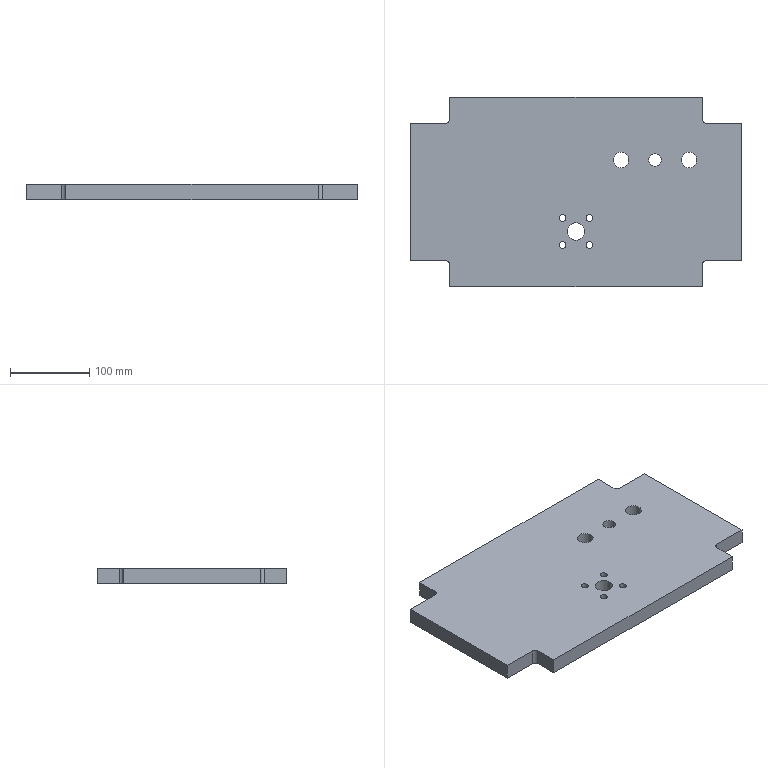Part | STEP file | Tube necking machine_id414_x_t | 1 solid | 26 faces | box 420 x 240 x 20 mm | volume 1855699 mm3 | plane 14 | cylinder 12 | commonest cylinder face diameters 8.5 x4 10 x4 20 x2 16 x1 22 x1